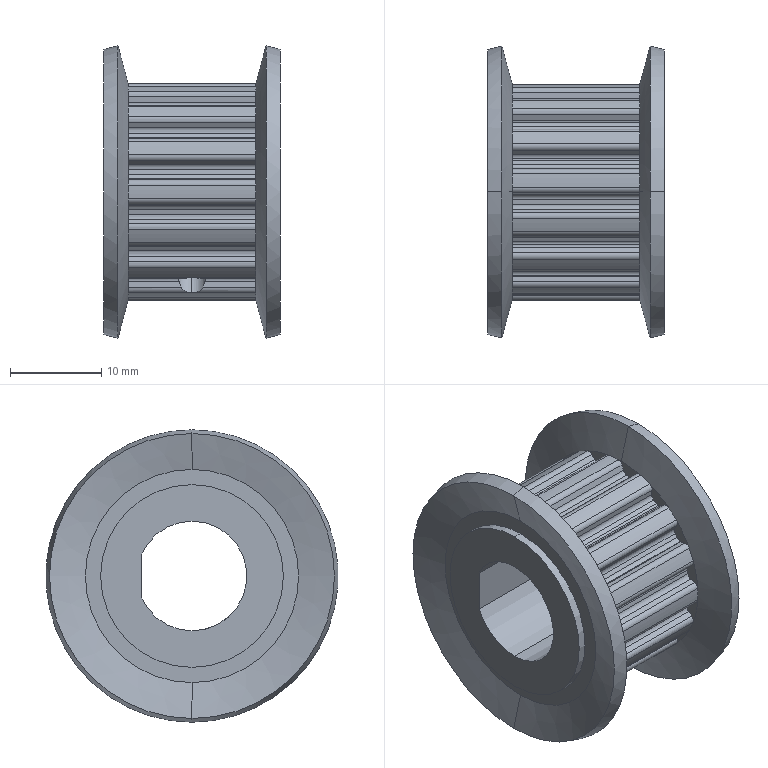Part | NX | features BREP 3 | 3 solids | 244 faces | box 19.302 x 32 x 32 mm | volume 6592 mm3 | cylinder 124 | plane 96 | cone 24 | commonest cylinder face diameters 1.22 x76 20.95 x17 23.75 x15 3.242 x4 4 x4 12 x4